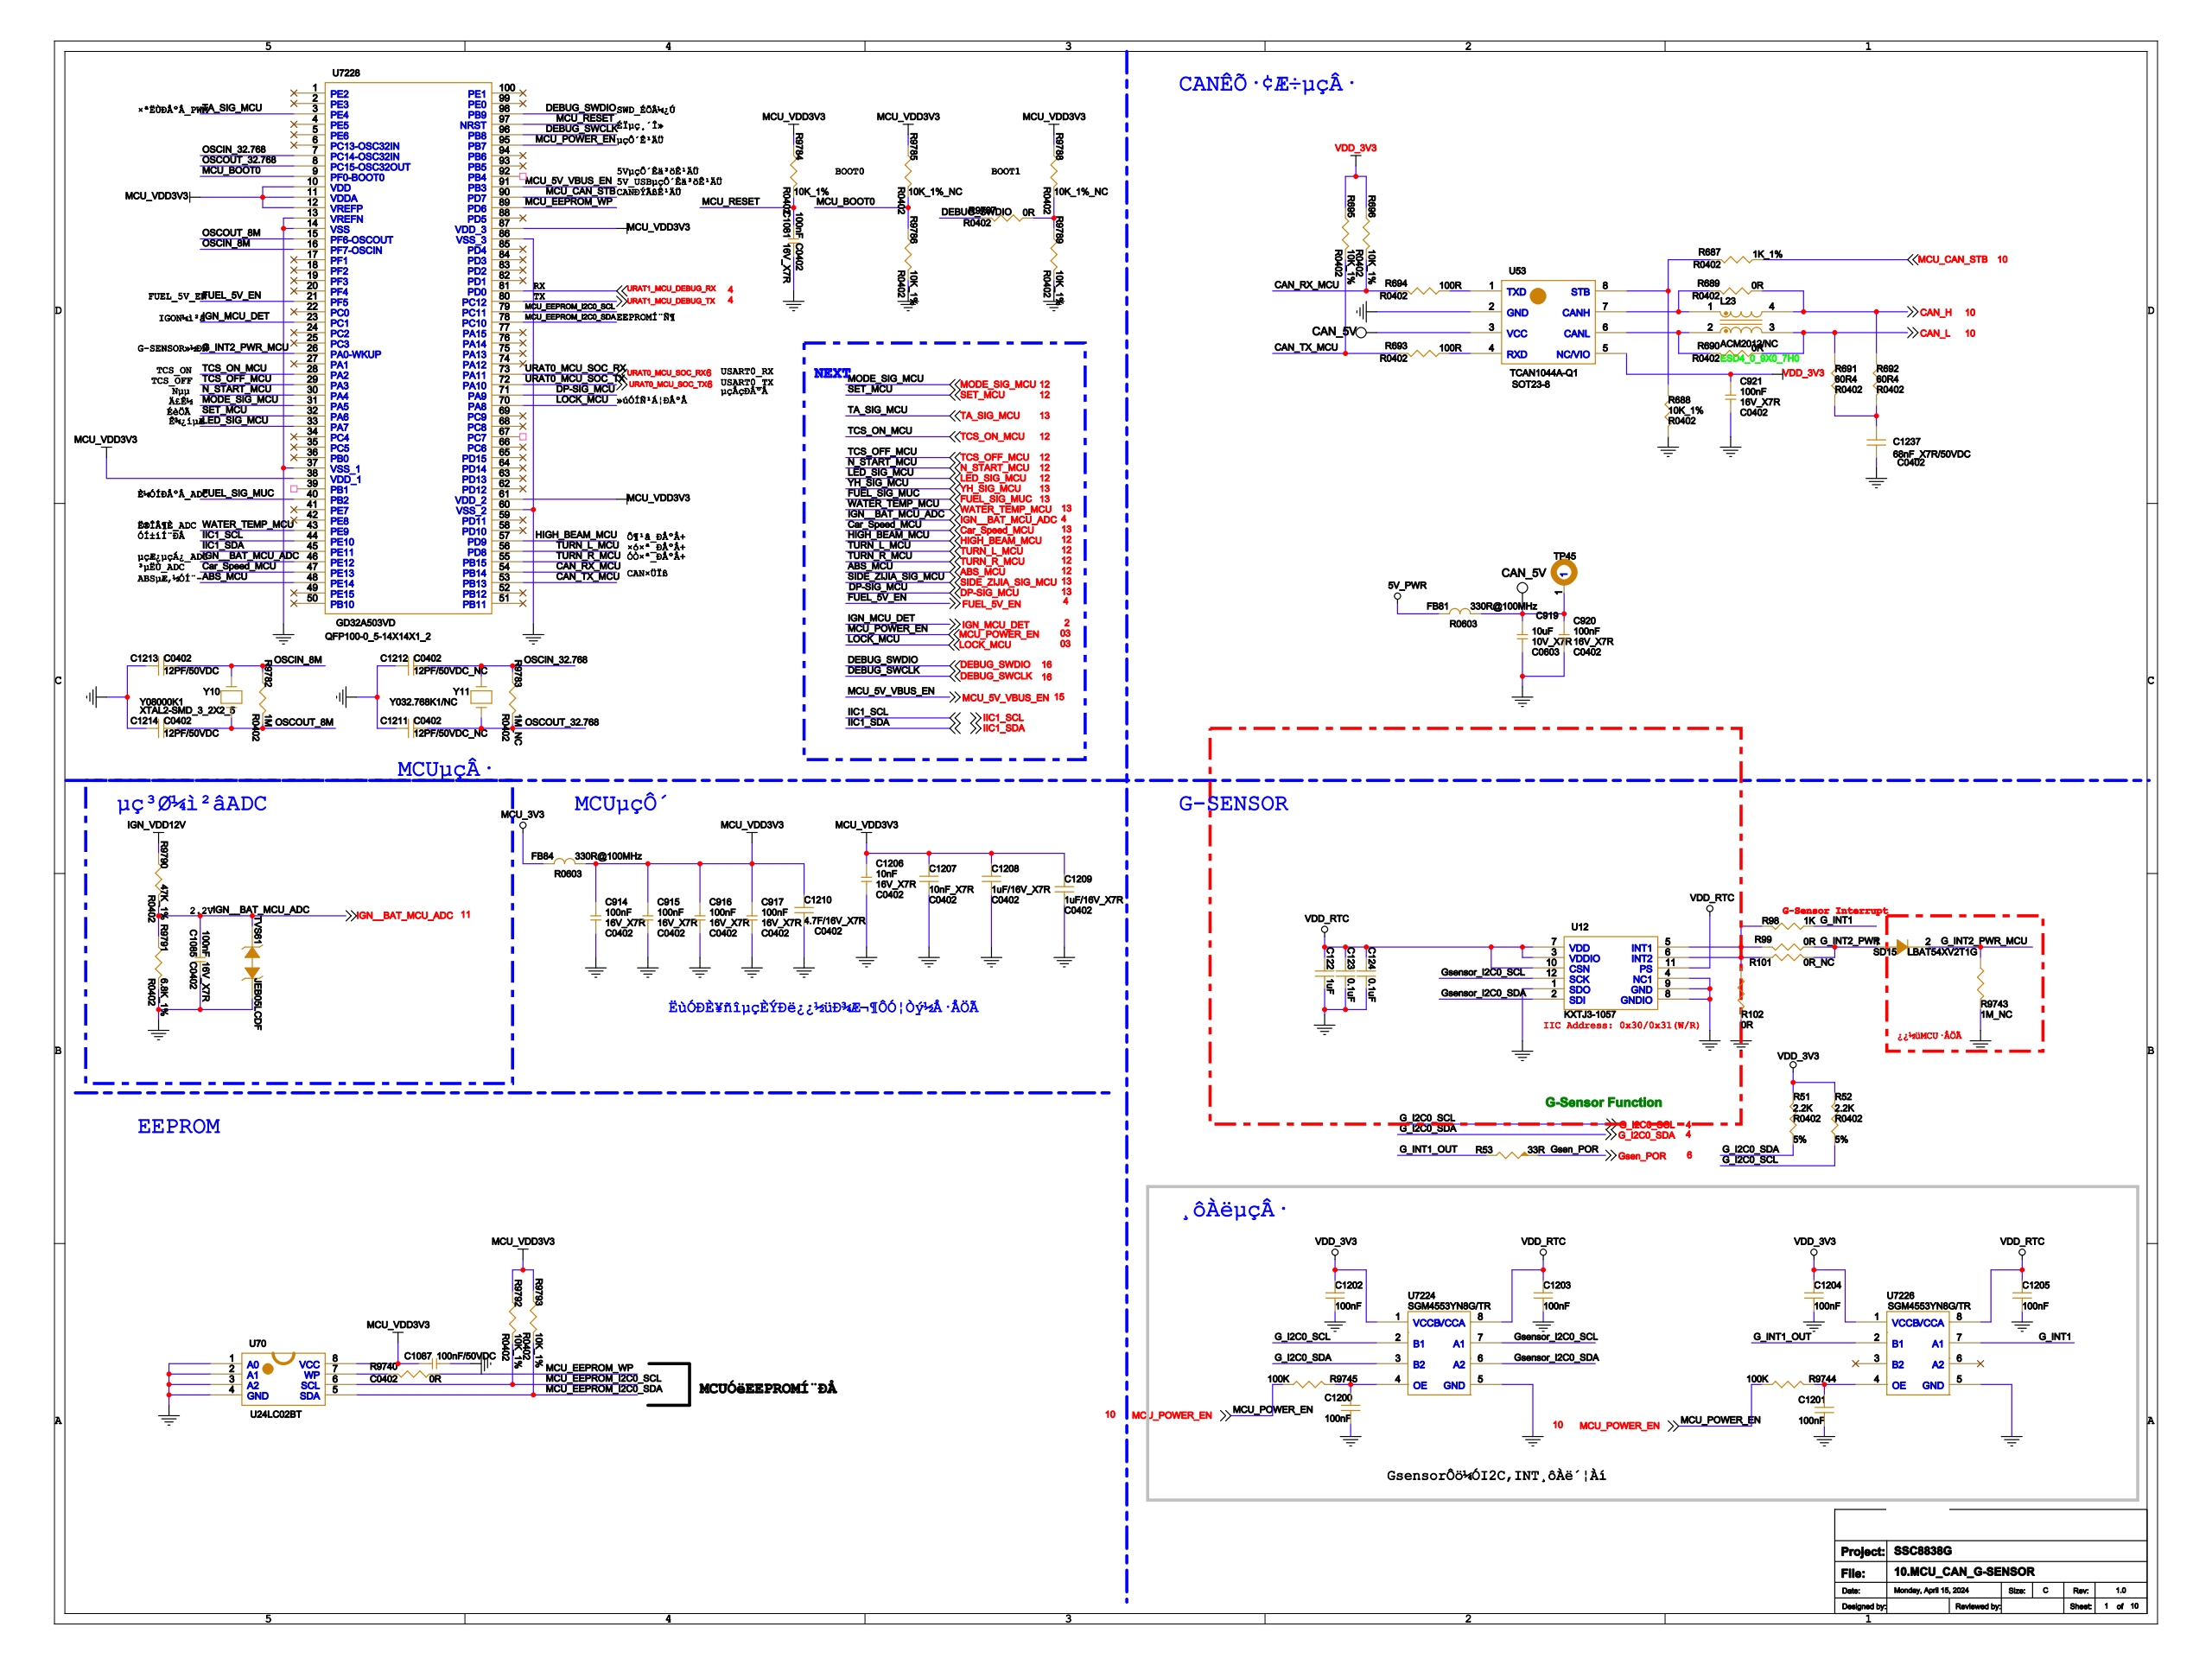Circuit board | Cadence Allegro | 958 parts | 601 nets | one sheet of the schematic
Parts on this sheet (reference | value | footprint):
C122 | 1uF | C0402
C123 | 0.1uF | C0402
C124 | 0.1uF | C0402
C914 | 100nF | C0402
C915 | 100nF | C0402
C916 | 100nF | C0402
C917 | 100nF | C0402
C919 | 10uF | C0603
C920 | 100nF | C0402
C921 | 100nF | C0402
C1081 | 100nF | C0402
C1085 | 100nF | C0402
C1087 | 100nF/50VDC | C0402
C1200 | 100nF | C0402
C1201 | 100nF | C0402
C1202 | 100nF | C0402
C1203 | 100nF | C0402
C1204 | 100nF | C0402
C1205 | 100nF | C0402
C1206 | 10nF | C0402
C1207 | 10nF_X7R | C0402
C1208 | 1uF/16V_X7R | C0402
C1209 | 1uF/16V_X7R | C0402
C1210 | 4.7F/16V_X7R | C0402
C1211 | 12PF/50VDC_NC | C0402
C1212 | 12PF/50VDC_NC | C0402
C1213 | 12PF/50VDC | C0402
C1214 | 12PF/50VDC | C0402
C1237 | 68nF_X7R/50VDC | C0402
FB81 | 330R@100MHz | R0603
FB84 | 330R@100MHz | R0603
L23 | ACM2012/NC | ESD4_0_9X0_7H0
R51 | 2.2K | R0402
R52 | 2.2K | R0402
R53 | 33R | R0402
R98 | 1K | R0402
R99 | 0R | R0402
R101 | 0R_NC | R0402
R102 | 0R | R0402
R687 | 1K_1% | R0402
R688 | 10K_1% | R0402
R689 | 0R | R0402
R690 | 0R | R0402
R691 | 60R4 | R0402
R692 | 60R4 | R0402
R693 | 100R | R0402
R694 | 100R | R0402
R695 | 10K_1% | R0402
R696 | 10K_1% | R0402
R9740 | 0R | R0402
R9743 | 1M_NC | R0402
R9744 | 100K | R0402
R9745 | 100K | R0402
R9782 | 1M | R0402
R9783 | 1M_NC | R0402
R9784 | 10K_1% | R0402
R9785 | 10K_1%_NC | R0402
R9786 | 10K_1% | R0402
R9787 | 0R | R0402
R9788 | 10K_1%_NC | R0402
R9789 | 10K_1% | R0402
R9790 | 47K_1% | R0402
R9791 | 6.8K_1% | R0402
R9792 | 10K_1% | R0402
R9793 | 10K_1% | R0402
SD15 | LBAT54XV2T1G | SOD_523
TP45 | HOLE | TP_0R50
TVS61 | JEB05LCDF | DFN1006
U12 | KXTJ3-1057 | LGA12-2X2-P0_5-H1
U53 | TCAN1044A-Q1 | SOT23-8
U70 | U24LC02BT | SOP8
U7224 | SGM4553YN8G/TR | SOT23-8
U7226 | SGM4553YN8G/TR | SOT23-8
U7228 | GD32A503VD | QFP100-0_5-14X14X1_2
Y10 | Y08000K1 | XTAL2-SMD_3_2X2_5
Y11 | Y032.768K1/NC | XTALS-SMD-3215
Nets of these parts (net: part-pin ...):
GND: C122-1 C123-1 C124-1 C914-1 C915-1 C916-1 C917-1 C919-1 C920-1 C921-1 C1081-1 C1085-1 C1087-1 C1200-2 C1201-2 C1202-2 C1203-2 C1204-2 C1205-2 C1206-1 C1207-2 C1208-2 C1209-2 C1210-2 C1211-1 C1212-1 C1213-1 C1214-1 C1237-1 R102-2 R688-2 R9743-2 R9786-2 R9789-2 R9791-2 TVS61-1 U12-1 U12-4 U12-8 U12-9 U53-2 U70-1 U70-2 U70-3 U70-4 U7224-5 U7226-5 U7228-13 U7228-14 U7228-37 U7228-60 U7228-86
5V_PWR: FB81-1
3V3_NORMAL: C921-2 C1202-1 C1204-1 R51-2 R52-2 R695-1 R696-1 U53-5 U7224-1 U7226-1
MCU_RESET: C1081-2 R9784-2 U7228-97
IGN__BAT_MCU_ADC: C1085-2 R9790-2 R9791-1 TVS61-2 U7228-46
MCU_VDD3V3: C914-2 C915-2 C916-2 C917-2 C1087-2 C1206-2 C1207-1 C1208-1 C1209-1 C1210-1 FB84-2 R9784-1 R9785-1 R9788-1 R9792-1 R9793-1 U70-8 U7228-10 U7228-11 U7228-12 U7228-38 U7228-61 U7228-87
CAN_5V: C919-2 C920-2 FB81-2 TP45-1 U53-3
N21416968: C1200-1 R9745-2 U7224-4
N21416847: C1201-1 R9744-2 U7226-4
VDD_RTC: C122-2 C123-2 C124-2 C1203-1 C1205-1 U12-3 U12-7 U12-10 U12-11 U7224-8 U7226-8
OSCOUT_32.768: C1211-2 R9783-2 Y11-1 U7228-8
OSCIN_32.768: C1212-2 R9783-1 Y11-2 U7228-7
OSCIN_8M: C1213-2 R9782-1 Y10-2 U7228-16
OSCOUT_8M: C1214-2 R9782-2 Y10-1 U7228-15
N21522793: C1237-2 R691-2 R692-2
IGN_VDD12V: R9790-1
MCU_POWER_EN: R9744-1 R9745-1 U7228-95
MCU_3V3: FB84-1
N21190026: L23-1 R689-2 U53-7
N21190049: L23-2 R690-2 U53-6
CAN_L: L23-3 R690-1 R691-1
CAN_H: L23-4 R689-1 R692-1
IIC1_SCL: U7228-44
IIC1_SDA: U7228-45
N21412962: R101-1 R102-1 U12-6
G_INT2_PWR: R99-1 R101-2 SD15-1
N21524844: R9787-1 R9788-2 R9789-1
DEBUG_SWDIO: R9787-2 U7228-98
N21412975: R98-2 R99-2 U12-5
MCU_CAN_STB: R687-1 U7228-90
N21190061: R687-2 R688-1 U53-8
G_I2C0_SCL: R52-1 U7224-2
G_I2C0_SDA: R51-1 U7224-3
GSEN_POR: R53-1
G_INT1_OUT: R53-2 U7226-2
CAN_TX_MCU: R693-2 R695-2 U7228-53
CAN_RX_MCU: R694-2 R696-2 U7228-54
MCU_BOOT0: R9785-2 R9786-1 U7228-9
MCU_EEPROM_I2C0_SCL: R9792-2 U70-6 U7228-79
MCU_EEPROM_I2C0_SDA: R9793-2 U70-5 U7228-78
N21191726: R693-1 U53-4
N21191767: R694-1 U53-1
ABS_MCU: U7228-48
HIGH_BEAM_MCU: U7228-57
TURN_R_MCU: U7228-55
TURN_L_MCU: U7228-56
N_START_MCU: U7228-30
TCS_ON_MCU: U7228-28
IGN_MCU_DET: U7228-23
TCS_OFF_MCU: U7228-29
TA_SIG_MCU: U7228-3
LED_SIG_MCU: U7228-33
FUEL_SIG_MUC: U7228-40
WATER_TEMP_MCU: U7228-43
DP-SIG_MCU: U7228-71
MCU_EEPROM_WP: R9740-1 U7228-89
N21411226: R9740-2 U70-7
LOCK_MCU: U7228-70
SET_MCU: U7228-32
MODE_SIG_MCU: U7228-31
DEBUG_SWCLK: U7228-96
URAT1_MCU_DEBUG_RX: U7228-81
URAT1_MCU_DEBUG_TX: U7228-80
MCU_5V_VBUS_EN: U7228-91
FUEL_5V_EN: U7228-21
G_INT2_PWR_MCU: R9743-1 SD15-2 U7228-26
G_INT1: R98-1 U7226-7
URAT0_MCU_SOC_RX: U7228-73
URAT0_MCU_SOC_TX: U7228-72
GSENSOR_I2C0_SCL: U12-12 U7224-7
GSENSOR_I2C0_SDA: U12-2 U7224-6